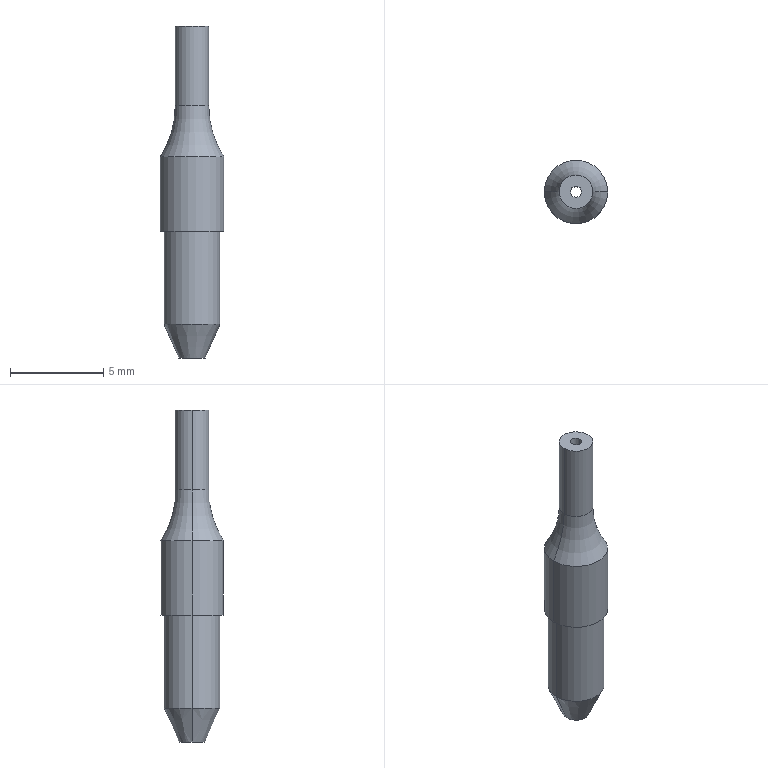Part | SolidWorks | features Boss 2, Chamfer 1, Cut 1, Extrusion 1, Fillet 1 | 1 solid | 15 faces | box 3.4 x 3.4 x 17.8 mm | volume 96.571 mm3 | cylinder 8 | plane 3 | torus 2 | cone 2 | commonest cylinder face diameters 0.6 x2 1.8 x2 3 x2 3.4 x2
STEP:
#1=CARTESIAN_POINT('',(1.7,0.,0.));
#2=VERTEX_POINT('',#1);
#3=CARTESIAN_POINT('',(-1.7,0.,0.));
#4=VERTEX_POINT('',#3);
#5=CARTESIAN_POINT('',(0.,0.,0.));
#6=DIRECTION('',(0.,0.,-1.));
#7=DIRECTION('',(-1.,0.,0.));
#8=AXIS2_PLACEMENT_3D('',#5,#6,#7);
#9=CIRCLE('',#8,1.7);
#10=EDGE_CURVE('',#2,#4,#9,.T.);
#11=ORIENTED_EDGE('',*,*,#10,.F.);
#12=CARTESIAN_POINT('',(0.9,0.,2.713));
#13=VERTEX_POINT('',#12);
#14=CARTESIAN_POINT('',(5.9,0.,2.713));
#15=DIRECTION('',(0.,1.,0.));
#16=DIRECTION('',(-1.,0.,0.));
#17=AXIS2_PLACEMENT_3D('',#14,#15,#16);
#18=CIRCLE('',#17,5.);
#19=EDGE_CURVE('',#2,#13,#18,.T.);
#20=ORIENTED_EDGE('',*,*,#19,.T.);
#21=CARTESIAN_POINT('',(-0.9,0.,2.713));
#22=VERTEX_POINT('',#21);
#23=CARTESIAN_POINT('',(0.,0.,2.713));
#24=DIRECTION('',(0.,0.,1.));
#25=DIRECTION('',(-1.,0.,0.));
#26=AXIS2_PLACEMENT_3D('',#23,#24,#25);
#27=CIRCLE('',#26,0.9);
#28=EDGE_CURVE('',#22,#13,#27,.T.);
#29=ORIENTED_EDGE('',*,*,#28,.F.);
#30=CARTESIAN_POINT('',(-5.9,0.,2.713));
#31=DIRECTION('',(0.,-1.,0.));
#32=DIRECTION('',(0.,0.,-1.));
#33=AXIS2_PLACEMENT_3D('',#30,#31,#32);
#34=CIRCLE('',#33,5.);
#35=EDGE_CURVE('',#4,#22,#34,.T.);
#36=ORIENTED_EDGE('',*,*,#35,.F.);
#37=EDGE_LOOP('',(#11,#20,#29,#36));
#38=FACE_OUTER_BOUND('',#37,.T.);
#39=CARTESIAN_POINT('',(0.,0.,2.713));
#40=DIRECTION('',(0.,0.,-1.));
#41=DIRECTION('',(-1.,0.,0.));
#42=AXIS2_PLACEMENT_3D('',#39,#40,#41);
#43=TOROIDAL_SURFACE('',#42,5.9,5.);
#44=ADVANCED_FACE('',(#38),#43,.F.);
#45=CARTESIAN_POINT('',(-0.3,0.,-10.8));
#46=VERTEX_POINT('',#45);
#47=CARTESIAN_POINT('',(0.3,0.,-10.8));
#48=VERTEX_POINT('',#47);
#49=CARTESIAN_POINT('',(0.,0.,-10.8));
#50=DIRECTION('',(0.,0.,1.));
#51=DIRECTION('',(1.,0.,0.));
#52=AXIS2_PLACEMENT_3D('',#49,#50,#51);
#53=CIRCLE('',#52,0.3);
#54=EDGE_CURVE('',#46,#48,#53,.T.);
#55=ORIENTED_EDGE('',*,*,#54,.F.);
#56=CARTESIAN_POINT('',(-0.3,0.,7.));
#57=VERTEX_POINT('',#56);
#58=CARTESIAN_POINT('',(-0.3,0.,-10.8));
#59=DIRECTION('',(0.,0.,1.));
#60=VECTOR('',#59,1000.);
#61=LINE('',#58,#60);
#62=EDGE_CURVE('',#46,#57,#61,.T.);
#63=ORIENTED_EDGE('',*,*,#62,.T.);
#64=CARTESIAN_POINT('',(0.3,0.,7.));
#65=VERTEX_POINT('',#64);
#66=CARTESIAN_POINT('',(0.,0.,7.));
#67=DIRECTION('',(0.,0.,1.));
#68=DIRECTION('',(1.,0.,0.));
#69=AXIS2_PLACEMENT_3D('',#66,#67,#68);
#70=CIRCLE('',#69,0.3);
#71=EDGE_CURVE('',#57,#65,#70,.T.);
#72=ORIENTED_EDGE('',*,*,#71,.T.);
#73=CARTESIAN_POINT('',(0.3,0.,-10.8));
#74=DIRECTION('',(0.,0.,1.));
#75=VECTOR('',#74,1000.);
#76=LINE('',#73,#75);
#77=EDGE_CURVE('',#48,#65,#76,.T.);
#78=ORIENTED_EDGE('',*,*,#77,.F.);
#79=EDGE_LOOP('',(#55,#63,#72,#78));
#80=FACE_OUTER_BOUND('',#79,.T.);
#81=CARTESIAN_POINT('',(0.,0.,-10.8));
#82=DIRECTION('',(0.,0.,1.));
#83=DIRECTION('',(1.,0.,0.));
#84=AXIS2_PLACEMENT_3D('',#81,#82,#83);
#85=CYLINDRICAL_SURFACE('',#84,0.3);
#86=ADVANCED_FACE('',(#80),#85,.F.);
#87=CARTESIAN_POINT('',(-0.7,0.,-10.8));
#88=VERTEX_POINT('',#87);
#89=CARTESIAN_POINT('',(0.7,0.,-10.8));
#90=VERTEX_POINT('',#89);
#91=CARTESIAN_POINT('',(0.,0.,-10.8));
#92=DIRECTION('',(0.,0.,-1.));
#93=DIRECTION('',(-1.,0.,0.));
#94=AXIS2_PLACEMENT_3D('',#91,#92,#93);
#95=CIRCLE('',#94,0.7);
#96=EDGE_CURVE('',#88,#90,#95,.T.);
#97=ORIENTED_EDGE('',*,*,#96,.F.);
#98=CARTESIAN_POINT('',(-1.5,0.,-9.));
#99=VERTEX_POINT('',#98);
#100=CARTESIAN_POINT('',(-0.7,0.,-10.8));
#101=DIRECTION('',(-0.4061,0.,0.9138));
#102=VECTOR('',#101,1000.);
#103=LINE('',#100,#102);
#104=EDGE_CURVE('',#88,#99,#103,.T.);
#105=ORIENTED_EDGE('',*,*,#104,.T.);
#106=CARTESIAN_POINT('',(1.5,0.,-9.));
#107=VERTEX_POINT('',#106);
#108=CARTESIAN_POINT('',(0.,0.,-9.));
#109=DIRECTION('',(0.,0.,1.));
#110=DIRECTION('',(-1.,0.,0.));
#111=AXIS2_PLACEMENT_3D('',#108,#109,#110);
#112=CIRCLE('',#111,1.5);
#113=EDGE_CURVE('',#107,#99,#112,.T.);
#114=ORIENTED_EDGE('',*,*,#113,.F.);
#115=CARTESIAN_POINT('',(0.7,0.,-10.8));
#116=DIRECTION('',(0.4061,0.,0.9138));
#117=VECTOR('',#116,1000.);
#118=LINE('',#115,#117);
#119=EDGE_CURVE('',#90,#107,#118,.T.);
#120=ORIENTED_EDGE('',*,*,#119,.F.);
#121=EDGE_LOOP('',(#97,#105,#114,#120));
#122=FACE_OUTER_BOUND('',#121,.T.);
#123=CARTESIAN_POINT('',(0.,0.,-10.8));
#124=DIRECTION('',(0.,0.,1.));
#125=DIRECTION('',(1.,0.,0.));
#126=AXIS2_PLACEMENT_3D('',#123,#124,#125);
#127=CONICAL_SURFACE('',#126,0.7,0.4182);
#128=ADVANCED_FACE('',(#122),#127,.T.);
#129=ORIENTED_EDGE('',*,*,#113,.T.);
#130=CARTESIAN_POINT('',(-1.5,0.,-4.));
#131=VERTEX_POINT('',#130);
#132=CARTESIAN_POINT('',(-1.5,0.,-10.8));
#133=DIRECTION('',(0.,0.,1.));
#134=VECTOR('',#133,1000.);
#135=LINE('',#132,#134);
#136=EDGE_CURVE('',#99,#131,#135,.T.);
#137=ORIENTED_EDGE('',*,*,#136,.T.);
#138=CARTESIAN_POINT('',(1.5,0.,-4.));
#139=VERTEX_POINT('',#138);
#140=CARTESIAN_POINT('',(0.,0.,-4.));
#141=DIRECTION('',(0.,0.,-1.));
#142=DIRECTION('',(-1.,0.,0.));
#143=AXIS2_PLACEMENT_3D('',#140,#141,#142);
#144=CIRCLE('',#143,1.5);
#145=EDGE_CURVE('',#131,#139,#144,.T.);
#146=ORIENTED_EDGE('',*,*,#145,.T.);
#147=CARTESIAN_POINT('',(1.5,0.,-10.8));
#148=DIRECTION('',(0.,0.,1.));
#149=VECTOR('',#148,1000.);
#150=LINE('',#147,#149);
#151=EDGE_CURVE('',#107,#139,#150,.T.);
#152=ORIENTED_EDGE('',*,*,#151,.F.);
#153=EDGE_LOOP('',(#129,#137,#146,#152));
#154=FACE_OUTER_BOUND('',#153,.T.);
#155=CARTESIAN_POINT('',(0.,0.,-10.8));
#156=DIRECTION('',(0.,0.,1.));
#157=DIRECTION('',(1.,0.,0.));
#158=AXIS2_PLACEMENT_3D('',#155,#156,#157);
#159=CYLINDRICAL_SURFACE('',#158,1.5);
#160=ADVANCED_FACE('',(#154),#159,.T.);
#161=CARTESIAN_POINT('',(-1.7,0.,-4.));
#162=VERTEX_POINT('',#161);
#163=CARTESIAN_POINT('',(1.7,0.,-4.));
#164=VERTEX_POINT('',#163);
#165=CARTESIAN_POINT('',(0.,0.,-4.));
#166=DIRECTION('',(0.,0.,-1.));
#167=DIRECTION('',(-1.,0.,0.));
#168=AXIS2_PLACEMENT_3D('',#165,#166,#167);
#169=CIRCLE('',#168,1.7);
#170=EDGE_CURVE('',#162,#164,#169,.T.);
#171=ORIENTED_EDGE('',*,*,#170,.F.);
#172=CARTESIAN_POINT('',(-1.7,0.,-4.));
#173=DIRECTION('',(0.,0.,1.));
#174=VECTOR('',#173,1000.);
#175=LINE('',#172,#174);
#176=EDGE_CURVE('',#162,#4,#175,.T.);
#177=ORIENTED_EDGE('',*,*,#176,.T.);
#178=CARTESIAN_POINT('',(0.,0.,0.));
#179=DIRECTION('',(0.,0.,-1.));
#180=DIRECTION('',(-1.,0.,0.));
#181=AXIS2_PLACEMENT_3D('',#178,#179,#180);
#182=CIRCLE('',#181,1.7);
#183=EDGE_CURVE('',#4,#2,#182,.T.);
#184=ORIENTED_EDGE('',*,*,#183,.T.);
#185=CARTESIAN_POINT('',(1.7,0.,-4.));
#186=DIRECTION('',(0.,0.,1.));
#187=VECTOR('',#186,1000.);
#188=LINE('',#185,#187);
#189=EDGE_CURVE('',#164,#2,#188,.T.);
#190=ORIENTED_EDGE('',*,*,#189,.F.);
#191=EDGE_LOOP('',(#171,#177,#184,#190));
#192=FACE_OUTER_BOUND('',#191,.T.);
#193=CARTESIAN_POINT('',(0.,0.,-4.));
#194=DIRECTION('',(0.,0.,1.));
#195=DIRECTION('',(1.,0.,0.));
#196=AXIS2_PLACEMENT_3D('',#193,#194,#195);
#197=CYLINDRICAL_SURFACE('',#196,1.7);
#198=ADVANCED_FACE('',(#192),#197,.T.);
#199=CARTESIAN_POINT('',(0.9,0.,7.));
#200=VERTEX_POINT('',#199);
#201=CARTESIAN_POINT('',(-0.9,0.,7.));
#202=VERTEX_POINT('',#201);
#203=CARTESIAN_POINT('',(0.,0.,7.));
#204=DIRECTION('',(0.,0.,1.));
#205=DIRECTION('',(1.,0.,0.));
#206=AXIS2_PLACEMENT_3D('',#203,#204,#205);
#207=CIRCLE('',#206,0.9);
#208=EDGE_CURVE('',#200,#202,#207,.T.);
#209=ORIENTED_EDGE('',*,*,#208,.F.);
#210=CARTESIAN_POINT('',(0.9,0.,7.));
#211=DIRECTION('',(0.,0.,-1.));
#212=VECTOR('',#211,1000.);
#213=LINE('',#210,#212);
#214=EDGE_CURVE('',#200,#13,#213,.T.);
#215=ORIENTED_EDGE('',*,*,#214,.T.);
#216=CARTESIAN_POINT('',(0.,0.,2.713));
#217=DIRECTION('',(0.,0.,1.));
#218=DIRECTION('',(-1.,0.,0.));
#219=AXIS2_PLACEMENT_3D('',#216,#217,#218);
#220=CIRCLE('',#219,0.9);
#221=EDGE_CURVE('',#13,#22,#220,.T.);
#222=ORIENTED_EDGE('',*,*,#221,.T.);
#223=CARTESIAN_POINT('',(-0.9,0.,7.));
#224=DIRECTION('',(0.,0.,-1.));
#225=VECTOR('',#224,1000.);
#226=LINE('',#223,#225);
#227=EDGE_CURVE('',#202,#22,#226,.T.);
#228=ORIENTED_EDGE('',*,*,#227,.F.);
#229=EDGE_LOOP('',(#209,#215,#222,#228));
#230=FACE_OUTER_BOUND('',#229,.T.);
#231=CARTESIAN_POINT('',(0.,0.,7.));
#232=DIRECTION('',(0.,0.,-1.));
#233=DIRECTION('',(-1.,0.,0.));
#234=AXIS2_PLACEMENT_3D('',#231,#232,#233);
#235=CYLINDRICAL_SURFACE('',#234,0.9);
#236=ADVANCED_FACE('',(#230),#235,.T.);
#237=CARTESIAN_POINT('',(0.,0.,-4.));
#238=DIRECTION('',(0.,0.,-1.));
#239=DIRECTION('',(-1.,0.,0.));
#240=AXIS2_PLACEMENT_3D('',#237,#238,#239);
#241=CIRCLE('',#240,1.7);
#242=EDGE_CURVE('',#164,#162,#241,.T.);
#243=ORIENTED_EDGE('',*,*,#242,.T.);
#244=ORIENTED_EDGE('',*,*,#170,.T.);
#245=EDGE_LOOP('',(#243,#244));
#246=FACE_OUTER_BOUND('',#245,.T.);
#247=CARTESIAN_POINT('',(0.,0.,-4.));
#248=DIRECTION('',(0.,0.,-1.));
#249=DIRECTION('',(-1.,0.,0.));
#250=AXIS2_PLACEMENT_3D('',#247,#248,#249);
#251=CIRCLE('',#250,1.5);
#252=EDGE_CURVE('',#139,#131,#251,.T.);
#253=ORIENTED_EDGE('',*,*,#252,.F.);
#254=ORIENTED_EDGE('',*,*,#145,.F.);
#255=EDGE_LOOP('',(#253,#254));
#256=FACE_BOUND('',#255,.T.);
#257=CARTESIAN_POINT('',(0.,0.,-4.));
#258=DIRECTION('',(0.,0.,-1.));
#259=DIRECTION('',(-1.,0.,0.));
#260=AXIS2_PLACEMENT_3D('',#257,#258,#259);
#261=PLANE('',#260);
#262=ADVANCED_FACE('',(#246,#256),#261,.T.);
#263=ORIENTED_EDGE('',*,*,#214,.F.);
#264=CARTESIAN_POINT('',(0.,0.,7.));
#265=DIRECTION('',(0.,0.,1.));
#266=DIRECTION('',(1.,0.,0.));
#267=AXIS2_PLACEMENT_3D('',#264,#265,#266);
#268=CIRCLE('',#267,0.9);
#269=EDGE_CURVE('',#202,#200,#268,.T.);
#270=ORIENTED_EDGE('',*,*,#269,.F.);
#271=ORIENTED_EDGE('',*,*,#227,.T.);
#272=ORIENTED_EDGE('',*,*,#28,.T.);
#273=EDGE_LOOP('',(#263,#270,#271,#272));
#274=FACE_OUTER_BOUND('',#273,.T.);
#275=CARTESIAN_POINT('',(0.,0.,7.));
#276=DIRECTION('',(0.,0.,-1.));
#277=DIRECTION('',(-1.,0.,0.));
#278=AXIS2_PLACEMENT_3D('',#275,#276,#277);
#279=CYLINDRICAL_SURFACE('',#278,0.9);
#280=ADVANCED_FACE('',(#274),#279,.T.);
#281=CARTESIAN_POINT('',(0.,0.,7.));
#282=DIRECTION('',(0.,0.,1.));
#283=DIRECTION('',(1.,0.,0.));
#284=AXIS2_PLACEMENT_3D('',#281,#282,#283);
#285=CIRCLE('',#284,0.3);
#286=EDGE_CURVE('',#65,#57,#285,.T.);
#287=ORIENTED_EDGE('',*,*,#286,.F.);
#288=ORIENTED_EDGE('',*,*,#71,.F.);
#289=EDGE_LOOP('',(#287,#288));
#290=FACE_BOUND('',#289,.T.);
#291=ORIENTED_EDGE('',*,*,#269,.T.);
#292=ORIENTED_EDGE('',*,*,#208,.T.);
#293=EDGE_LOOP('',(#291,#292));
#294=FACE_OUTER_BOUND('',#293,.T.);
#295=CARTESIAN_POINT('',(0.,0.,7.));
#296=DIRECTION('',(0.,0.,1.));
#297=DIRECTION('',(1.,0.,0.));
#298=AXIS2_PLACEMENT_3D('',#295,#296,#297);
#299=PLANE('',#298);
#300=ADVANCED_FACE('',(#290,#294),#299,.T.);
#301=ORIENTED_EDGE('',*,*,#176,.F.);
#302=ORIENTED_EDGE('',*,*,#242,.F.);
#303=ORIENTED_EDGE('',*,*,#189,.T.);
#304=ORIENTED_EDGE('',*,*,#10,.T.);
#305=EDGE_LOOP('',(#301,#302,#303,#304));
#306=FACE_OUTER_BOUND('',#305,.T.);
#307=CARTESIAN_POINT('',(0.,0.,-4.));
#308=DIRECTION('',(0.,0.,1.));
#309=DIRECTION('',(1.,0.,0.));
#310=AXIS2_PLACEMENT_3D('',#307,#308,#309);
#311=CYLINDRICAL_SURFACE('',#310,1.7);
#312=ADVANCED_FACE('',(#306),#311,.T.);
#313=ORIENTED_EDGE('',*,*,#136,.F.);
#314=CARTESIAN_POINT('',(0.,0.,-9.));
#315=DIRECTION('',(0.,0.,1.));
#316=DIRECTION('',(-1.,0.,0.));
#317=AXIS2_PLACEMENT_3D('',#314,#315,#316);
#318=CIRCLE('',#317,1.5);
#319=EDGE_CURVE('',#99,#107,#318,.T.);
#320=ORIENTED_EDGE('',*,*,#319,.T.);
#321=ORIENTED_EDGE('',*,*,#151,.T.);
#322=ORIENTED_EDGE('',*,*,#252,.T.);
#323=EDGE_LOOP('',(#313,#320,#321,#322));
#324=FACE_OUTER_BOUND('',#323,.T.);
#325=CARTESIAN_POINT('',(0.,0.,-10.8));
#326=DIRECTION('',(0.,0.,1.));
#327=DIRECTION('',(1.,0.,0.));
#328=AXIS2_PLACEMENT_3D('',#325,#326,#327);
#329=CYLINDRICAL_SURFACE('',#328,1.5);
#330=ADVANCED_FACE('',(#324),#329,.T.);
#331=CARTESIAN_POINT('',(0.,0.,-10.8));
#332=DIRECTION('',(0.,0.,1.));
#333=DIRECTION('',(1.,0.,0.));
#334=AXIS2_PLACEMENT_3D('',#331,#332,#333);
#335=CIRCLE('',#334,0.3);
#336=EDGE_CURVE('',#48,#46,#335,.T.);
#337=ORIENTED_EDGE('',*,*,#336,.T.);
#338=ORIENTED_EDGE('',*,*,#54,.T.);
#339=EDGE_LOOP('',(#337,#338));
#340=FACE_BOUND('',#339,.T.);
#341=CARTESIAN_POINT('',(0.,0.,-10.8));
#342=DIRECTION('',(0.,0.,-1.));
#343=DIRECTION('',(-1.,0.,0.));
#344=AXIS2_PLACEMENT_3D('',#341,#342,#343);
#345=CIRCLE('',#344,0.7);
#346=EDGE_CURVE('',#90,#88,#345,.T.);
#347=ORIENTED_EDGE('',*,*,#346,.T.);
#348=ORIENTED_EDGE('',*,*,#96,.T.);
#349=EDGE_LOOP('',(#347,#348));
#350=FACE_OUTER_BOUND('',#349,.T.);
#351=CARTESIAN_POINT('',(0.,0.,-10.8));
#352=DIRECTION('',(0.,0.,-1.));
#353=DIRECTION('',(-1.,0.,0.));
#354=AXIS2_PLACEMENT_3D('',#351,#352,#353);
#355=PLANE('',#354);
#356=ADVANCED_FACE('',(#340,#350),#355,.T.);
#357=ORIENTED_EDGE('',*,*,#104,.F.);
#358=ORIENTED_EDGE('',*,*,#346,.F.);
#359=ORIENTED_EDGE('',*,*,#119,.T.);
#360=ORIENTED_EDGE('',*,*,#319,.F.);
#361=EDGE_LOOP('',(#357,#358,#359,#360));
#362=FACE_OUTER_BOUND('',#361,.T.);
#363=CARTESIAN_POINT('',(0.,0.,-10.8));
#364=DIRECTION('',(0.,0.,1.));
#365=DIRECTION('',(1.,0.,0.));
#366=AXIS2_PLACEMENT_3D('',#363,#364,#365);
#367=CONICAL_SURFACE('',#366,0.7,0.4182);
#368=ADVANCED_FACE('',(#362),#367,.T.);
#369=ORIENTED_EDGE('',*,*,#62,.F.);
#370=ORIENTED_EDGE('',*,*,#336,.F.);
#371=ORIENTED_EDGE('',*,*,#77,.T.);
#372=ORIENTED_EDGE('',*,*,#286,.T.);
#373=EDGE_LOOP('',(#369,#370,#371,#372));
#374=FACE_OUTER_BOUND('',#373,.T.);
#375=CARTESIAN_POINT('',(0.,0.,-10.8));
#376=DIRECTION('',(0.,0.,1.));
#377=DIRECTION('',(1.,0.,0.));
#378=AXIS2_PLACEMENT_3D('',#375,#376,#377);
#379=CYLINDRICAL_SURFACE('',#378,0.3);
#380=ADVANCED_FACE('',(#374),#379,.F.);
#381=ORIENTED_EDGE('',*,*,#19,.F.);
#382=ORIENTED_EDGE('',*,*,#183,.F.);
#383=ORIENTED_EDGE('',*,*,#35,.T.);
#384=ORIENTED_EDGE('',*,*,#221,.F.);
#385=EDGE_LOOP('',(#381,#382,#383,#384));
#386=FACE_OUTER_BOUND('',#385,.T.);
#387=CARTESIAN_POINT('',(0.,0.,2.713));
#388=DIRECTION('',(0.,0.,-1.));
#389=DIRECTION('',(-1.,0.,0.));
#390=AXIS2_PLACEMENT_3D('',#387,#388,#389);
#391=TOROIDAL_SURFACE('',#390,5.9,5.);
#392=ADVANCED_FACE('',(#386),#391,.F.);
#393=CLOSED_SHELL('',(#44,#86,#128,#160,#198,#236,#262,#280,#300,#312,#330,#356,#368,#380,#392));
#394=MANIFOLD_SOLID_BREP('',#393);
#395=CARTESIAN_POINT('',(0.,0.,0.));
#396=DIRECTION('',(0.,0.,1.));
#397=DIRECTION('',(1.,0.,0.));
#398=AXIS2_PLACEMENT_3D('',#395,#396,#397);
#399=(LENGTH_UNIT()NAMED_UNIT(*)SI_UNIT(.MILLI.,.METRE.));
#400=UNCERTAINTY_MEASURE_WITH_UNIT(LENGTH_MEASURE(0.00001),#399,'','');
#401=(NAMED_UNIT(*)PLANE_ANGLE_UNIT()SI_UNIT($,.RADIAN.));
#402=(NAMED_UNIT(*)SI_UNIT($,.STERADIAN.)SOLID_ANGLE_UNIT());
#403=(GEOMETRIC_REPRESENTATION_CONTEXT(3)GLOBAL_UNCERTAINTY_ASSIGNED_CONTEXT((#400))GLOBAL_UNIT_ASSIGNED_CONTEXT((#399,#401,#402))REPRESENTATION_CONTEXT('',''));
#404=ADVANCED_BREP_SHAPE_REPRESENTATION('',(#394,#398),#403);